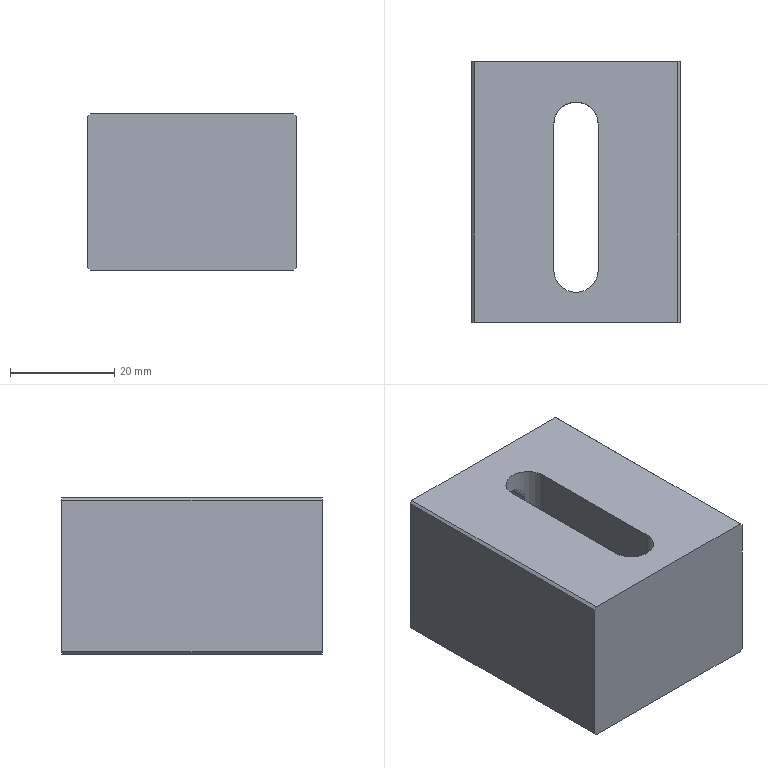CAM job | NX | 3-axis milling | part box 40 x 50 x 30 mm | stock box 45 x 55 x 35 mm
Tools:
number,name,description,diameter,corner_radius,flute_length,length,flutes
6,D6,平底铣刀-粗,6.0,0.0,25.0,75.0,2
9,D10,平底铣刀-粗,10.0,0.0,35.0,75.0,2
7,D6-J,平底铣刀-精,6.0,0.0,25.0,75.0,2
1,D80R0.8_FLYCUTTER,圆鼻刀-粗,80.0,0.8,50.0,75.0,2
1,D80R0.8_FLYCUTTER-J,圆鼻刀-精,80.0,0.8,50.0,75.0,2
2,D6_CHAMFERTOOL,倒角刀,6.0,0.0,3.0,25.0,2
Operations:
program,operation,operation_type,tool,method,geometry_group,spindle_rpm,surface_speed,feed_per_tooth,feed_cut,feed_plunge,cut_length_mm,path_length_mm,cut_time_min,machine_time_min
B,BOTTOMWALL_FLYFACE_ONEPASSROUGH_COPY,VolumeBased25DMillingOperation,D80R0.8_FLYCUTTER,LAYER-ROUGH-DEPTHK-STEPG,W-B,2800.0,703.696,0.5357,3000.0,100.0,1423.746,3215.967,0.4746,0.6538
B,BOTTOMWALL_FLYFACE_ONEPASSFINISH_COPY,VolumeBased25DMillingOperation,D80R0.8_FLYCUTTER-J,SIDEFINISH-DEPTHK-STEPG,W-B,4000.0,1005.28,0.125,1000.0,100.0,157.998,253.998,0.158,0.1676
B,PLANEDEBURR6X45L_COPY,SurfaceContour,D6_CHAMFERTOOL,CLIMBFACE_CHAMFER-DEPTH0-STEPG,W-B,6500.0,122.519,0.1154,1500.0,100.0,166.644,391.657,0.1111,0.1336
B,BOTTOMWALL_CHAMFER_COPY_1,VolumeBased25DMillingOperation,D6_CHAMFERTOOL,CLIMBFACE_CHAMFER-DEPTH0-STEPG,W-B,6500.0,122.519,0.1154,1500.0,100.0,124.592,367.192,0.0831,0.1073
A,TOPFACE,FaceMilling,D80R0.8_FLYCUTTER,SIDEFINISH-DEPTHK-STEPG,W-A,4500.0,1385.0,0.1667,1500.0,100.0,144.0,240.0,0.096,0.1056
A,PROFILE_ROUGH_2,VolumeBased25DMillingOperation,D10,METHOD,W-A,8000.0,251.327,0.375,6000.0,80.0,8483.326,8611.826,1.414,1.427
A,THROUGHSLOT_ROUGH_1,VolumeBased25DMillingOperation,D6,METHOD,W-A,9000.0,169.646,0.1389,2500.0,100.0,3984.839,4113.839,1.594,1.607
A,SELECTBODYONLY,SurfaceContour,D6_CHAMFERTOOL,METHOD,W-A,8000.0,150.796,0.1875,3000.0,100.0,181.313,548.875,0.0604,0.0972
A,BOTTOMWALL_CHAMFER_COPY,VolumeBased25DMillingOperation,D6_CHAMFERTOOL,CLIMBFACE_CHAMFER-DEPTH0-STEPG,W-A,6500.0,122.519,0.1154,1500.0,100.0,124.592,367.192,0.0831,0.1073
A,SLOT_FINISH_1,VolumeBased25DMillingOperation,D6-J,METHOD,W-A,8000.0,150.796,0.0375,600.0,100.0,330.411,545.011,0.5507,0.5721
A,PROFILE_SEMIFINISH_2,VolumeBased25DMillingOperation,D6-J,METHOD,W-A,9000.0,169.646,0.0667,1200.0,100.0,610.824,1032.865,0.509,0.5512